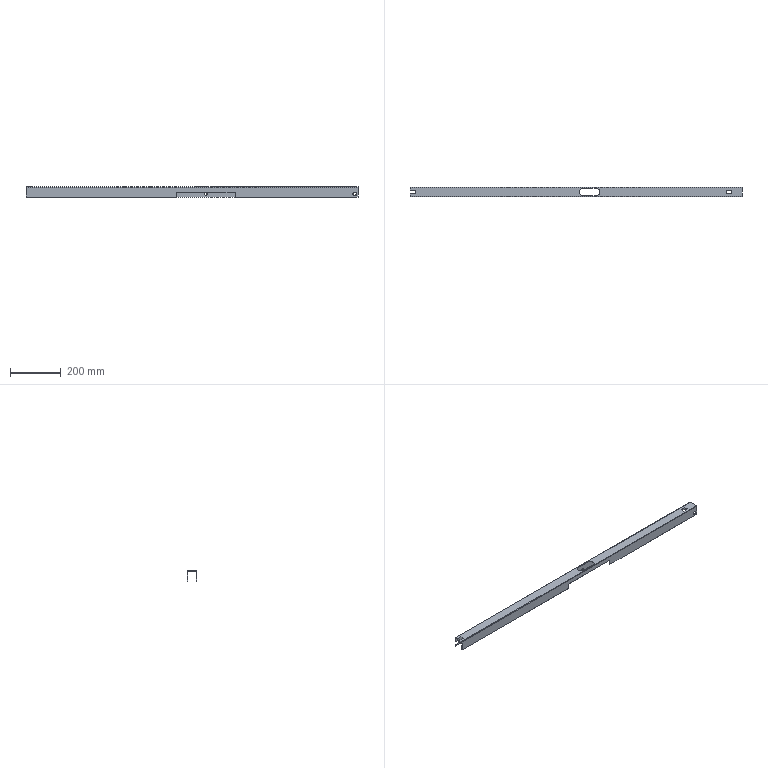Part | SolidWorks | features Cut 4, ICE 2, SMBaseFlange 2, FlatPattern 1, SheetMetal 1 | 1 solid | 68 faces | box 1302 x 38 x 40 mm | volume 208795 mm3 | plane 48 | cylinder 20 | commonest cylinder face diameters 10 x10 0.4 x2 3.4 x2 11 x2 15 x2 30 x2